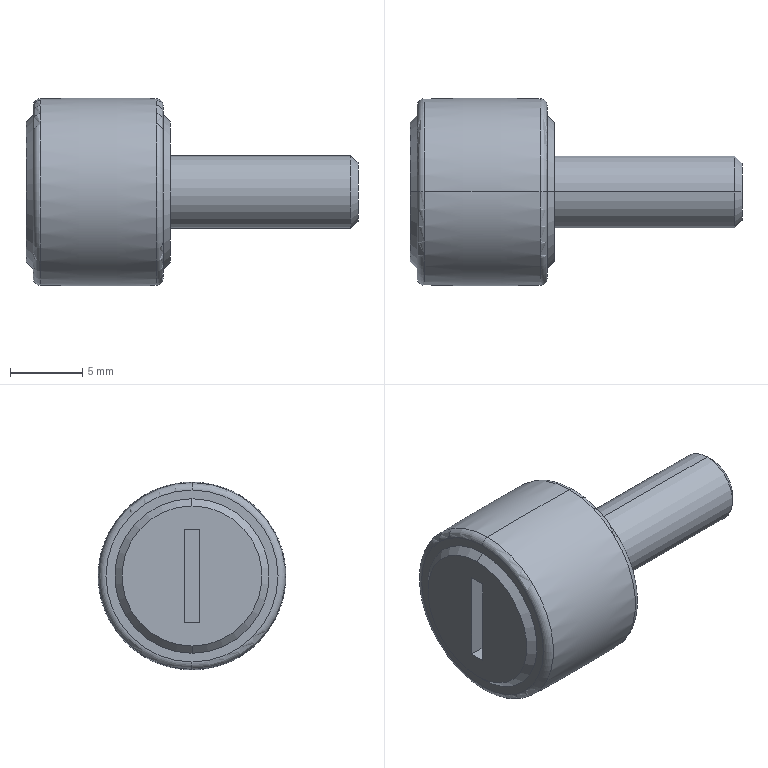Part | SolidWorks | features ICE 1, Revolution 1 | 1 solid | 24 faces | box 23 x 13 x 13 mm | volume 1507 mm3 | plane 10 | cone 6 | torus 6 | cylinder 2 | commonest cylinder face diameters 5 x2
STEP:
#1=CARTESIAN_POINT('',(13.,0.,2.01));
#2=VERTEX_POINT('',#1);
#3=CARTESIAN_POINT('',(13.,0.,-2.01));
#4=VERTEX_POINT('',#3);
#5=CARTESIAN_POINT('',(13.,0.,0.));
#6=DIRECTION('',(-1.,0.,0.));
#7=DIRECTION('',(0.,0.,1.));
#8=AXIS2_PLACEMENT_3D('',#5,#6,#7);
#9=CIRCLE('',#8,2.01);
#10=EDGE_CURVE('',#2,#4,#9,.T.);
#11=ORIENTED_EDGE('',*,*,#10,.T.);
#12=CARTESIAN_POINT('',(12.509,0.,-2.5));
#13=VERTEX_POINT('',#12);
#14=CARTESIAN_POINT('',(13.,0.,-2.01));
#15=DIRECTION('',(-0.7071,0.,-0.7071));
#16=VECTOR('',#15,1000.);
#17=LINE('',#14,#16);
#18=EDGE_CURVE('',#4,#13,#17,.T.);
#19=ORIENTED_EDGE('',*,*,#18,.T.);
#20=CARTESIAN_POINT('',(12.509,0.,2.5));
#21=VERTEX_POINT('',#20);
#22=CARTESIAN_POINT('',(12.509,0.,0.));
#23=DIRECTION('',(-1.,0.,0.));
#24=DIRECTION('',(0.,0.,1.));
#25=AXIS2_PLACEMENT_3D('',#22,#23,#24);
#26=CIRCLE('',#25,2.5);
#27=EDGE_CURVE('',#21,#13,#26,.T.);
#28=ORIENTED_EDGE('',*,*,#27,.F.);
#29=CARTESIAN_POINT('',(13.,0.,2.01));
#30=DIRECTION('',(-0.7071,0.,0.7071));
#31=VECTOR('',#30,1000.);
#32=LINE('',#29,#31);
#33=EDGE_CURVE('',#2,#21,#32,.T.);
#34=ORIENTED_EDGE('',*,*,#33,.F.);
#35=EDGE_LOOP('',(#11,#19,#28,#34));
#36=FACE_OUTER_BOUND('',#35,.T.);
#37=CARTESIAN_POINT('',(13.,0.,0.));
#38=DIRECTION('',(-1.,0.,0.));
#39=DIRECTION('',(0.,0.,1.));
#40=AXIS2_PLACEMENT_3D('',#37,#38,#39);
#41=CONICAL_SURFACE('',#40,2.01,0.7854);
#42=ADVANCED_FACE('',(#36),#41,.T.);
#43=ORIENTED_EDGE('',*,*,#27,.T.);
#44=CARTESIAN_POINT('',(0.,0.,-2.5));
#45=VERTEX_POINT('',#44);
#46=CARTESIAN_POINT('',(13.,0.,-2.5));
#47=DIRECTION('',(-1.,0.,0.));
#48=VECTOR('',#47,1000.);
#49=LINE('',#46,#48);
#50=EDGE_CURVE('',#13,#45,#49,.T.);
#51=ORIENTED_EDGE('',*,*,#50,.T.);
#52=CARTESIAN_POINT('',(0.,0.,2.5));
#53=VERTEX_POINT('',#52);
#54=CARTESIAN_POINT('',(0.,0.,0.));
#55=DIRECTION('',(-1.,0.,0.));
#56=DIRECTION('',(0.,0.,1.));
#57=AXIS2_PLACEMENT_3D('',#54,#55,#56);
#58=CIRCLE('',#57,2.5);
#59=EDGE_CURVE('',#53,#45,#58,.T.);
#60=ORIENTED_EDGE('',*,*,#59,.F.);
#61=CARTESIAN_POINT('',(13.,0.,2.5));
#62=DIRECTION('',(-1.,0.,0.));
#63=VECTOR('',#62,1000.);
#64=LINE('',#61,#63);
#65=EDGE_CURVE('',#21,#53,#64,.T.);
#66=ORIENTED_EDGE('',*,*,#65,.F.);
#67=EDGE_LOOP('',(#43,#51,#60,#66));
#68=FACE_OUTER_BOUND('',#67,.T.);
#69=CARTESIAN_POINT('',(13.,0.,0.));
#70=DIRECTION('',(-1.,0.,0.));
#71=DIRECTION('',(0.,0.,1.));
#72=AXIS2_PLACEMENT_3D('',#69,#70,#71);
#73=CYLINDRICAL_SURFACE('',#72,2.5);
#74=ADVANCED_FACE('',(#68),#73,.T.);
#75=CARTESIAN_POINT('',(0.,0.,4.85));
#76=VERTEX_POINT('',#75);
#77=CARTESIAN_POINT('',(0.,0.,-4.85));
#78=VERTEX_POINT('',#77);
#79=CARTESIAN_POINT('',(0.,0.,0.));
#80=DIRECTION('',(-1.,0.,0.));
#81=DIRECTION('',(0.,0.,1.));
#82=AXIS2_PLACEMENT_3D('',#79,#80,#81);
#83=CIRCLE('',#82,4.85);
#84=EDGE_CURVE('',#76,#78,#83,.T.);
#85=ORIENTED_EDGE('',*,*,#84,.T.);
#86=CARTESIAN_POINT('',(-0.5,0.,-5.35));
#87=VERTEX_POINT('',#86);
#88=CARTESIAN_POINT('',(0.,0.,-4.85));
#89=DIRECTION('',(-0.7071,0.,-0.7071));
#90=VECTOR('',#89,1000.);
#91=LINE('',#88,#90);
#92=EDGE_CURVE('',#78,#87,#91,.T.);
#93=ORIENTED_EDGE('',*,*,#92,.T.);
#94=CARTESIAN_POINT('',(-0.5,0.,5.35));
#95=VERTEX_POINT('',#94);
#96=CARTESIAN_POINT('',(-0.5,0.,0.));
#97=DIRECTION('',(-1.,0.,0.));
#98=DIRECTION('',(0.,0.,1.));
#99=AXIS2_PLACEMENT_3D('',#96,#97,#98);
#100=CIRCLE('',#99,5.35);
#101=EDGE_CURVE('',#95,#87,#100,.T.);
#102=ORIENTED_EDGE('',*,*,#101,.F.);
#103=CARTESIAN_POINT('',(0.,0.,4.85));
#104=DIRECTION('',(-0.7071,0.,0.7071));
#105=VECTOR('',#104,1000.);
#106=LINE('',#103,#105);
#107=EDGE_CURVE('',#76,#95,#106,.T.);
#108=ORIENTED_EDGE('',*,*,#107,.F.);
#109=EDGE_LOOP('',(#85,#93,#102,#108));
#110=FACE_OUTER_BOUND('',#109,.T.);
#111=CARTESIAN_POINT('',(0.,0.,0.));
#112=DIRECTION('',(-1.,0.,0.));
#113=DIRECTION('',(0.,0.,1.));
#114=AXIS2_PLACEMENT_3D('',#111,#112,#113);
#115=CONICAL_SURFACE('',#114,4.85,0.7854);
#116=ADVANCED_FACE('',(#110),#115,.T.);
#117=CARTESIAN_POINT('',(-0.5,0.,5.975));
#118=VERTEX_POINT('',#117);
#119=CARTESIAN_POINT('',(-0.5,0.,-5.975));
#120=VERTEX_POINT('',#119);
#121=CARTESIAN_POINT('',(-0.5,0.,0.));
#122=DIRECTION('',(-1.,0.,0.));
#123=DIRECTION('',(0.,0.,1.));
#124=AXIS2_PLACEMENT_3D('',#121,#122,#123);
#125=CIRCLE('',#124,5.975);
#126=EDGE_CURVE('',#118,#120,#125,.T.);
#127=ORIENTED_EDGE('',*,*,#126,.T.);
#128=CARTESIAN_POINT('',(-0.993,0.,-6.475));
#129=VERTEX_POINT('',#128);
#130=CARTESIAN_POINT('',(-1.,0.,-5.975));
#131=DIRECTION('',(0.,1.,0.));
#132=DIRECTION('',(0.,0.,1.));
#133=AXIS2_PLACEMENT_3D('',#130,#131,#132);
#134=CIRCLE('',#133,0.5);
#135=EDGE_CURVE('',#120,#129,#134,.T.);
#136=ORIENTED_EDGE('',*,*,#135,.T.);
#137=CARTESIAN_POINT('',(-0.993,0.,6.475));
#138=VERTEX_POINT('',#137);
#139=CARTESIAN_POINT('',(-0.993,0.,0.));
#140=DIRECTION('',(-1.,0.,0.));
#141=DIRECTION('',(0.,0.,1.));
#142=AXIS2_PLACEMENT_3D('',#139,#140,#141);
#143=CIRCLE('',#142,6.475);
#144=EDGE_CURVE('',#138,#129,#143,.T.);
#145=ORIENTED_EDGE('',*,*,#144,.F.);
#146=CARTESIAN_POINT('',(-1.,0.,5.975));
#147=DIRECTION('',(0.,-1.,0.));
#148=DIRECTION('',(0.,0.,-1.));
#149=AXIS2_PLACEMENT_3D('',#146,#147,#148);
#150=CIRCLE('',#149,0.5);
#151=EDGE_CURVE('',#118,#138,#150,.T.);
#152=ORIENTED_EDGE('',*,*,#151,.F.);
#153=EDGE_LOOP('',(#127,#136,#145,#152));
#154=FACE_OUTER_BOUND('',#153,.T.);
#155=CARTESIAN_POINT('',(-1.,0.,0.));
#156=DIRECTION('',(-1.,0.,0.));
#157=DIRECTION('',(0.,0.,1.));
#158=AXIS2_PLACEMENT_3D('',#155,#156,#157);
#159=TOROIDAL_SURFACE('',#158,5.975,0.5);
#160=ADVANCED_FACE('',(#154),#159,.T.);
#161=ORIENTED_EDGE('',*,*,#144,.T.);
#162=CARTESIAN_POINT('',(-9.009,0.,-6.459));
#163=VERTEX_POINT('',#162);
#164=CARTESIAN_POINT('',(-4.5,0.,243.5));
#165=DIRECTION('',(0.,1.,0.));
#166=DIRECTION('',(0.,0.,1.));
#167=AXIS2_PLACEMENT_3D('',#164,#165,#166);
#168=CIRCLE('',#167,250.);
#169=EDGE_CURVE('',#129,#163,#168,.T.);
#170=ORIENTED_EDGE('',*,*,#169,.T.);
#171=CARTESIAN_POINT('',(-9.009,0.,6.459));
#172=VERTEX_POINT('',#171);
#173=CARTESIAN_POINT('',(-9.009,0.,0.));
#174=DIRECTION('',(-1.,0.,0.));
#175=DIRECTION('',(0.,0.,1.));
#176=AXIS2_PLACEMENT_3D('',#173,#174,#175);
#177=CIRCLE('',#176,6.459);
#178=EDGE_CURVE('',#172,#163,#177,.T.);
#179=ORIENTED_EDGE('',*,*,#178,.F.);
#180=CARTESIAN_POINT('',(-4.5,0.,-243.5));
#181=DIRECTION('',(0.,-1.,0.));
#182=DIRECTION('',(0.,0.,-1.));
#183=AXIS2_PLACEMENT_3D('',#180,#181,#182);
#184=CIRCLE('',#183,250.);
#185=EDGE_CURVE('',#138,#172,#184,.T.);
#186=ORIENTED_EDGE('',*,*,#185,.F.);
#187=EDGE_LOOP('',(#161,#170,#179,#186));
#188=FACE_OUTER_BOUND('',#187,.T.);
#189=CARTESIAN_POINT('',(-4.5,0.,0.));
#190=DIRECTION('',(-1.,0.,0.));
#191=DIRECTION('',(0.,0.,1.));
#192=AXIS2_PLACEMENT_3D('',#189,#190,#191);
#193=TOROIDAL_SURFACE('',#192,-243.5,250.);
#194=ADVANCED_FACE('',(#188),#193,.T.);
#195=ORIENTED_EDGE('',*,*,#178,.T.);
#196=CARTESIAN_POINT('',(-9.5,0.,-5.959));
#197=VERTEX_POINT('',#196);
#198=CARTESIAN_POINT('',(-9.,0.,-5.959));
#199=DIRECTION('',(0.,1.,0.));
#200=DIRECTION('',(0.,0.,1.));
#201=AXIS2_PLACEMENT_3D('',#198,#199,#200);
#202=CIRCLE('',#201,0.5);
#203=EDGE_CURVE('',#163,#197,#202,.T.);
#204=ORIENTED_EDGE('',*,*,#203,.T.);
#205=CARTESIAN_POINT('',(-9.5,0.,5.959));
#206=VERTEX_POINT('',#205);
#207=CARTESIAN_POINT('',(-9.5,0.,0.));
#208=DIRECTION('',(-1.,0.,0.));
#209=DIRECTION('',(0.,0.,1.));
#210=AXIS2_PLACEMENT_3D('',#207,#208,#209);
#211=CIRCLE('',#210,5.959);
#212=EDGE_CURVE('',#206,#197,#211,.T.);
#213=ORIENTED_EDGE('',*,*,#212,.F.);
#214=CARTESIAN_POINT('',(-9.,0.,5.959));
#215=DIRECTION('',(0.,-1.,0.));
#216=DIRECTION('',(0.,0.,-1.));
#217=AXIS2_PLACEMENT_3D('',#214,#215,#216);
#218=CIRCLE('',#217,0.5);
#219=EDGE_CURVE('',#172,#206,#218,.T.);
#220=ORIENTED_EDGE('',*,*,#219,.F.);
#221=EDGE_LOOP('',(#195,#204,#213,#220));
#222=FACE_OUTER_BOUND('',#221,.T.);
#223=CARTESIAN_POINT('',(-9.,0.,0.));
#224=DIRECTION('',(-1.,0.,0.));
#225=DIRECTION('',(0.,0.,1.));
#226=AXIS2_PLACEMENT_3D('',#223,#224,#225);
#227=TOROIDAL_SURFACE('',#226,5.959,0.5);
#228=ADVANCED_FACE('',(#222),#227,.T.);
#229=CARTESIAN_POINT('',(-10.,0.,4.85));
#230=VERTEX_POINT('',#229);
#231=CARTESIAN_POINT('',(-10.,0.,-4.85));
#232=VERTEX_POINT('',#231);
#233=CARTESIAN_POINT('',(-10.,0.,0.));
#234=DIRECTION('',(-1.,0.,0.));
#235=DIRECTION('',(0.,0.,1.));
#236=AXIS2_PLACEMENT_3D('',#233,#234,#235);
#237=CIRCLE('',#236,4.85);
#238=EDGE_CURVE('',#230,#232,#237,.T.);
#239=ORIENTED_EDGE('',*,*,#238,.F.);
#240=CARTESIAN_POINT('',(-9.5,0.,5.35));
#241=VERTEX_POINT('',#240);
#242=CARTESIAN_POINT('',(-9.5,0.,5.35));
#243=DIRECTION('',(0.7071,0.,0.7071));
#244=VECTOR('',#243,1000.);
#245=LINE('',#242,#244);
#246=EDGE_CURVE('',#230,#241,#245,.T.);
#247=ORIENTED_EDGE('',*,*,#246,.T.);
#248=CARTESIAN_POINT('',(-9.5,0.,-5.35));
#249=VERTEX_POINT('',#248);
#250=CARTESIAN_POINT('',(-9.5,0.,0.));
#251=DIRECTION('',(-1.,0.,0.));
#252=DIRECTION('',(0.,0.,1.));
#253=AXIS2_PLACEMENT_3D('',#250,#251,#252);
#254=CIRCLE('',#253,5.35);
#255=EDGE_CURVE('',#241,#249,#254,.T.);
#256=ORIENTED_EDGE('',*,*,#255,.T.);
#257=CARTESIAN_POINT('',(-9.5,0.,-5.35));
#258=DIRECTION('',(0.7071,0.,-0.7071));
#259=VECTOR('',#258,1000.);
#260=LINE('',#257,#259);
#261=EDGE_CURVE('',#232,#249,#260,.T.);
#262=ORIENTED_EDGE('',*,*,#261,.F.);
#263=EDGE_LOOP('',(#239,#247,#256,#262));
#264=FACE_OUTER_BOUND('',#263,.T.);
#265=CARTESIAN_POINT('',(-9.5,0.,0.));
#266=DIRECTION('',(1.,0.,0.));
#267=DIRECTION('',(0.,0.,-1.));
#268=AXIS2_PLACEMENT_3D('',#265,#266,#267);
#269=CONICAL_SURFACE('',#268,5.35,0.7854);
#270=ADVANCED_FACE('',(#264),#269,.T.);
#271=CARTESIAN_POINT('',(-10.,-0.5417,3.25));
#272=VERTEX_POINT('',#271);
#273=CARTESIAN_POINT('',(-10.,0.5417,3.25));
#274=VERTEX_POINT('',#273);
#275=CARTESIAN_POINT('',(-10.,-0.5417,3.25));
#276=DIRECTION('',(0.,1.,0.));
#277=VECTOR('',#276,1000.);
#278=LINE('',#275,#277);
#279=EDGE_CURVE('',#272,#274,#278,.T.);
#280=ORIENTED_EDGE('',*,*,#279,.F.);
#281=CARTESIAN_POINT('',(-10.,-0.5417,-3.25));
#282=VERTEX_POINT('',#281);
#283=CARTESIAN_POINT('',(-10.,-0.5417,-3.25));
#284=DIRECTION('',(0.,0.,1.));
#285=VECTOR('',#284,1000.);
#286=LINE('',#283,#285);
#287=EDGE_CURVE('',#282,#272,#286,.T.);
#288=ORIENTED_EDGE('',*,*,#287,.F.);
#289=CARTESIAN_POINT('',(-10.,0.5417,-3.25));
#290=VERTEX_POINT('',#289);
#291=CARTESIAN_POINT('',(-10.,0.5417,-3.25));
#292=DIRECTION('',(0.,-1.,0.));
#293=VECTOR('',#292,1000.);
#294=LINE('',#291,#293);
#295=EDGE_CURVE('',#290,#282,#294,.T.);
#296=ORIENTED_EDGE('',*,*,#295,.F.);
#297=CARTESIAN_POINT('',(-10.,0.5417,3.25));
#298=DIRECTION('',(0.,0.,-1.));
#299=VECTOR('',#298,1000.);
#300=LINE('',#297,#299);
#301=EDGE_CURVE('',#274,#290,#300,.T.);
#302=ORIENTED_EDGE('',*,*,#301,.F.);
#303=EDGE_LOOP('',(#280,#288,#296,#302));
#304=FACE_BOUND('',#303,.T.);
#305=CARTESIAN_POINT('',(-10.,0.,0.));
#306=DIRECTION('',(-1.,0.,0.));
#307=DIRECTION('',(0.,0.,1.));
#308=AXIS2_PLACEMENT_3D('',#305,#306,#307);
#309=CIRCLE('',#308,4.85);
#310=EDGE_CURVE('',#232,#230,#309,.T.);
#311=ORIENTED_EDGE('',*,*,#310,.T.);
#312=ORIENTED_EDGE('',*,*,#238,.T.);
#313=EDGE_LOOP('',(#311,#312));
#314=FACE_OUTER_BOUND('',#313,.T.);
#315=CARTESIAN_POINT('',(-10.,0.,0.));
#316=DIRECTION('',(1.,0.,0.));
#317=DIRECTION('',(0.,0.,-1.));
#318=AXIS2_PLACEMENT_3D('',#315,#316,#317);
#319=PLANE('',#318);
#320=ADVANCED_FACE('',(#304,#314),#319,.F.);
#321=ORIENTED_EDGE('',*,*,#246,.F.);
#322=ORIENTED_EDGE('',*,*,#310,.F.);
#323=ORIENTED_EDGE('',*,*,#261,.T.);
#324=CARTESIAN_POINT('',(-9.5,0.,0.));
#325=DIRECTION('',(-1.,0.,0.));
#326=DIRECTION('',(0.,0.,1.));
#327=AXIS2_PLACEMENT_3D('',#324,#325,#326);
#328=CIRCLE('',#327,5.35);
#329=EDGE_CURVE('',#249,#241,#328,.T.);
#330=ORIENTED_EDGE('',*,*,#329,.T.);
#331=EDGE_LOOP('',(#321,#322,#323,#330));
#332=FACE_OUTER_BOUND('',#331,.T.);
#333=CARTESIAN_POINT('',(-9.5,0.,0.));
#334=DIRECTION('',(1.,0.,0.));
#335=DIRECTION('',(0.,0.,-1.));
#336=AXIS2_PLACEMENT_3D('',#333,#334,#335);
#337=CONICAL_SURFACE('',#336,5.35,0.7854);
#338=ADVANCED_FACE('',(#332),#337,.T.);
#339=ORIENTED_EDGE('',*,*,#329,.F.);
#340=ORIENTED_EDGE('',*,*,#255,.F.);
#341=EDGE_LOOP('',(#339,#340));
#342=FACE_BOUND('',#341,.T.);
#343=ORIENTED_EDGE('',*,*,#212,.T.);
#344=CARTESIAN_POINT('',(-9.5,0.,0.));
#345=DIRECTION('',(-1.,0.,0.));
#346=DIRECTION('',(0.,0.,1.));
#347=AXIS2_PLACEMENT_3D('',#344,#345,#346);
#348=CIRCLE('',#347,5.959);
#349=EDGE_CURVE('',#197,#206,#348,.T.);
#350=ORIENTED_EDGE('',*,*,#349,.T.);
#351=EDGE_LOOP('',(#343,#350));
#352=FACE_OUTER_BOUND('',#351,.T.);
#353=CARTESIAN_POINT('',(-9.5,5.35,0.));
#354=DIRECTION('',(1.,0.,0.));
#355=DIRECTION('',(0.,0.,-1.));
#356=AXIS2_PLACEMENT_3D('',#353,#354,#355);
#357=PLANE('',#356);
#358=ADVANCED_FACE('',(#342,#352),#357,.F.);
#359=ORIENTED_EDGE('',*,*,#203,.F.);
#360=CARTESIAN_POINT('',(-9.009,0.,0.));
#361=DIRECTION('',(-1.,0.,0.));
#362=DIRECTION('',(0.,0.,1.));
#363=AXIS2_PLACEMENT_3D('',#360,#361,#362);
#364=CIRCLE('',#363,6.459);
#365=EDGE_CURVE('',#163,#172,#364,.T.);
#366=ORIENTED_EDGE('',*,*,#365,.T.);
#367=ORIENTED_EDGE('',*,*,#219,.T.);
#368=ORIENTED_EDGE('',*,*,#349,.F.);
#369=EDGE_LOOP('',(#359,#366,#367,#368));
#370=FACE_OUTER_BOUND('',#369,.T.);
#371=CARTESIAN_POINT('',(-9.,0.,0.));
#372=DIRECTION('',(-1.,0.,0.));
#373=DIRECTION('',(0.,0.,1.));
#374=AXIS2_PLACEMENT_3D('',#371,#372,#373);
#375=TOROIDAL_SURFACE('',#374,5.959,0.5);
#376=ADVANCED_FACE('',(#370),#375,.T.);
#377=ORIENTED_EDGE('',*,*,#169,.F.);
#378=CARTESIAN_POINT('',(-0.993,0.,0.));
#379=DIRECTION('',(-1.,0.,0.));
#380=DIRECTION('',(0.,0.,1.));
#381=AXIS2_PLACEMENT_3D('',#378,#379,#380);
#382=CIRCLE('',#381,6.475);
#383=EDGE_CURVE('',#129,#138,#382,.T.);
#384=ORIENTED_EDGE('',*,*,#383,.T.);
#385=ORIENTED_EDGE('',*,*,#185,.T.);
#386=ORIENTED_EDGE('',*,*,#365,.F.);
#387=EDGE_LOOP('',(#377,#384,#385,#386));
#388=FACE_OUTER_BOUND('',#387,.T.);
#389=CARTESIAN_POINT('',(-4.5,0.,0.));
#390=DIRECTION('',(-1.,0.,0.));
#391=DIRECTION('',(0.,0.,1.));
#392=AXIS2_PLACEMENT_3D('',#389,#390,#391);
#393=TOROIDAL_SURFACE('',#392,-243.5,250.);
#394=ADVANCED_FACE('',(#388),#393,.T.);
#395=ORIENTED_EDGE('',*,*,#135,.F.);
#396=CARTESIAN_POINT('',(-0.5,0.,0.));
#397=DIRECTION('',(-1.,0.,0.));
#398=DIRECTION('',(0.,0.,1.));
#399=AXIS2_PLACEMENT_3D('',#396,#397,#398);
#400=CIRCLE('',#399,5.975);
#401=EDGE_CURVE('',#120,#118,#400,.T.);
#402=ORIENTED_EDGE('',*,*,#401,.T.);
#403=ORIENTED_EDGE('',*,*,#151,.T.);
#404=ORIENTED_EDGE('',*,*,#383,.F.);
#405=EDGE_LOOP('',(#395,#402,#403,#404));
#406=FACE_OUTER_BOUND('',#405,.T.);
#407=CARTESIAN_POINT('',(-1.,0.,0.));
#408=DIRECTION('',(-1.,0.,0.));
#409=DIRECTION('',(0.,0.,1.));
#410=AXIS2_PLACEMENT_3D('',#407,#408,#409);
#411=TOROIDAL_SURFACE('',#410,5.975,0.5);
#412=ADVANCED_FACE('',(#406),#411,.T.);
#413=ORIENTED_EDGE('',*,*,#126,.F.);
#414=ORIENTED_EDGE('',*,*,#401,.F.);
#415=EDGE_LOOP('',(#413,#414));
#416=FACE_OUTER_BOUND('',#415,.T.);
#417=ORIENTED_EDGE('',*,*,#101,.T.);
#418=CARTESIAN_POINT('',(-0.5,0.,0.));
#419=DIRECTION('',(-1.,0.,0.));
#420=DIRECTION('',(0.,0.,1.));
#421=AXIS2_PLACEMENT_3D('',#418,#419,#420);
#422=CIRCLE('',#421,5.35);
#423=EDGE_CURVE('',#87,#95,#422,.T.);
#424=ORIENTED_EDGE('',*,*,#423,.T.);
#425=EDGE_LOOP('',(#417,#424));
#426=FACE_BOUND('',#425,.T.);
#427=CARTESIAN_POINT('',(-0.5,5.975,0.));
#428=DIRECTION('',(-1.,0.,0.));
#429=DIRECTION('',(0.,0.,1.));
#430=AXIS2_PLACEMENT_3D('',#427,#428,#429);
#431=PLANE('',#430);
#432=ADVANCED_FACE('',(#416,#426),#431,.F.);
#433=ORIENTED_EDGE('',*,*,#92,.F.);
#434=CARTESIAN_POINT('',(0.,0.,0.));
#435=DIRECTION('',(-1.,0.,0.));
#436=DIRECTION('',(0.,0.,1.));
#437=AXIS2_PLACEMENT_3D('',#434,#435,#436);
#438=CIRCLE('',#437,4.85);
#439=EDGE_CURVE('',#78,#76,#438,.T.);
#440=ORIENTED_EDGE('',*,*,#439,.T.);
#441=ORIENTED_EDGE('',*,*,#107,.T.);
#442=ORIENTED_EDGE('',*,*,#423,.F.);
#443=EDGE_LOOP('',(#433,#440,#441,#442));
#444=FACE_OUTER_BOUND('',#443,.T.);
#445=CARTESIAN_POINT('',(0.,0.,0.));
#446=DIRECTION('',(-1.,0.,0.));
#447=DIRECTION('',(0.,0.,1.));
#448=AXIS2_PLACEMENT_3D('',#445,#446,#447);
#449=CONICAL_SURFACE('',#448,4.85,0.7854);
#450=ADVANCED_FACE('',(#444),#449,.T.);
#451=ORIENTED_EDGE('',*,*,#84,.F.);
#452=ORIENTED_EDGE('',*,*,#439,.F.);
#453=EDGE_LOOP('',(#451,#452));
#454=FACE_OUTER_BOUND('',#453,.T.);
#455=ORIENTED_EDGE('',*,*,#59,.T.);
#456=CARTESIAN_POINT('',(0.,0.,0.));
#457=DIRECTION('',(-1.,0.,0.));
#458=DIRECTION('',(0.,0.,1.));
#459=AXIS2_PLACEMENT_3D('',#456,#457,#458);
#460=CIRCLE('',#459,2.5);
#461=EDGE_CURVE('',#45,#53,#460,.T.);
#462=ORIENTED_EDGE('',*,*,#461,.T.);
#463=EDGE_LOOP('',(#455,#462));
#464=FACE_BOUND('',#463,.T.);
#465=CARTESIAN_POINT('',(0.,4.85,0.));
#466=DIRECTION('',(-1.,0.,0.));
#467=DIRECTION('',(0.,0.,1.));
#468=AXIS2_PLACEMENT_3D('',#465,#466,#467);
#469=PLANE('',#468);
#470=ADVANCED_FACE('',(#454,#464),#469,.F.);
#471=ORIENTED_EDGE('',*,*,#50,.F.);
#472=CARTESIAN_POINT('',(12.509,0.,0.));
#473=DIRECTION('',(-1.,0.,0.));
#474=DIRECTION('',(0.,0.,1.));
#475=AXIS2_PLACEMENT_3D('',#472,#473,#474);
#476=CIRCLE('',#475,2.5);
#477=EDGE_CURVE('',#13,#21,#476,.T.);
#478=ORIENTED_EDGE('',*,*,#477,.T.);
#479=ORIENTED_EDGE('',*,*,#65,.T.);
#480=ORIENTED_EDGE('',*,*,#461,.F.);
#481=EDGE_LOOP('',(#471,#478,#479,#480));
#482=FACE_OUTER_BOUND('',#481,.T.);
#483=CARTESIAN_POINT('',(13.,0.,0.));
#484=DIRECTION('',(-1.,0.,0.));
#485=DIRECTION('',(0.,0.,1.));
#486=AXIS2_PLACEMENT_3D('',#483,#484,#485);
#487=CYLINDRICAL_SURFACE('',#486,2.5);
#488=ADVANCED_FACE('',(#482),#487,.T.);
#489=ORIENTED_EDGE('',*,*,#18,.F.);
#490=CARTESIAN_POINT('',(13.,0.,0.));
#491=DIRECTION('',(-1.,0.,0.));
#492=DIRECTION('',(0.,0.,1.));
#493=AXIS2_PLACEMENT_3D('',#490,#491,#492);
#494=CIRCLE('',#493,2.01);
#495=EDGE_CURVE('',#4,#2,#494,.T.);
#496=ORIENTED_EDGE('',*,*,#495,.T.);
#497=ORIENTED_EDGE('',*,*,#33,.T.);
#498=ORIENTED_EDGE('',*,*,#477,.F.);
#499=EDGE_LOOP('',(#489,#496,#497,#498));
#500=FACE_OUTER_BOUND('',#499,.T.);
#501=CARTESIAN_POINT('',(13.,0.,0.));
#502=DIRECTION('',(-1.,0.,0.));
#503=DIRECTION('',(0.,0.,1.));
#504=AXIS2_PLACEMENT_3D('',#501,#502,#503);
#505=CONICAL_SURFACE('',#504,2.01,0.7854);
#506=ADVANCED_FACE('',(#500),#505,.T.);
#507=ORIENTED_EDGE('',*,*,#10,.F.);
#508=ORIENTED_EDGE('',*,*,#495,.F.);
#509=EDGE_LOOP('',(#507,#508));
#510=FACE_OUTER_BOUND('',#509,.T.);
#511=CARTESIAN_POINT('',(13.,2.01,0.));
#512=DIRECTION('',(-1.,0.,0.));
#513=DIRECTION('',(0.,0.,1.));
#514=AXIS2_PLACEMENT_3D('',#511,#512,#513);
#515=PLANE('',#514);
#516=ADVANCED_FACE('',(#510),#515,.F.);
#517=ORIENTED_EDGE('',*,*,#287,.T.);
#518=CARTESIAN_POINT('',(-8.,-0.5417,3.25));
#519=VERTEX_POINT('',#518);
#520=CARTESIAN_POINT('',(-8.,-0.5417,3.25));
#521=DIRECTION('',(-1.,0.,0.));
#522=VECTOR('',#521,1000.);
#523=LINE('',#520,#522);
#524=EDGE_CURVE('',#519,#272,#523,.T.);
#525=ORIENTED_EDGE('',*,*,#524,.F.);
#526=CARTESIAN_POINT('',(-8.,-0.5417,-3.25));
#527=VERTEX_POINT('',#526);
#528=CARTESIAN_POINT('',(-8.,-0.5417,-3.25));
#529=DIRECTION('',(0.,0.,1.));
#530=VECTOR('',#529,1000.);
#531=LINE('',#528,#530);
#532=EDGE_CURVE('',#527,#519,#531,.T.);
#533=ORIENTED_EDGE('',*,*,#532,.F.);
#534=CARTESIAN_POINT('',(-8.,-0.5417,-3.25));
#535=DIRECTION('',(-1.,0.,0.));
#536=VECTOR('',#535,1000.);
#537=LINE('',#534,#536);
#538=EDGE_CURVE('',#527,#282,#537,.T.);
#539=ORIENTED_EDGE('',*,*,#538,.T.);
#540=EDGE_LOOP('',(#517,#525,#533,#539));
#541=FACE_OUTER_BOUND('',#540,.T.);
#542=CARTESIAN_POINT('',(-8.,-0.5417,-3.25));
#543=DIRECTION('',(0.,-1.,0.));
#544=DIRECTION('',(0.,0.,-1.));
#545=AXIS2_PLACEMENT_3D('',#542,#543,#544);
#546=PLANE('',#545);
#547=ADVANCED_FACE('',(#541),#546,.F.);
#548=ORIENTED_EDGE('',*,*,#295,.T.);
#549=ORIENTED_EDGE('',*,*,#538,.F.);
#550=CARTESIAN_POINT('',(-8.,0.5417,-3.25));
#551=VERTEX_POINT('',#550);
#552=CARTESIAN_POINT('',(-8.,0.5417,-3.25));
#553=DIRECTION('',(0.,-1.,0.));
#554=VECTOR('',#553,1000.);
#555=LINE('',#552,#554);
#556=EDGE_CURVE('',#551,#527,#555,.T.);
#557=ORIENTED_EDGE('',*,*,#556,.F.);
#558=CARTESIAN_POINT('',(-8.,0.5417,-3.25));
#559=DIRECTION('',(-1.,0.,0.));
#560=VECTOR('',#559,1000.);
#561=LINE('',#558,#560);
#562=EDGE_CURVE('',#551,#290,#561,.T.);
#563=ORIENTED_EDGE('',*,*,#562,.T.);
#564=EDGE_LOOP('',(#548,#549,#557,#563));
#565=FACE_OUTER_BOUND('',#564,.T.);
#566=CARTESIAN_POINT('',(-8.,0.5417,-3.25));
#567=DIRECTION('',(0.,0.,-1.));
#568=DIRECTION('',(-1.,0.,0.));
#569=AXIS2_PLACEMENT_3D('',#566,#567,#568);
#570=PLANE('',#569);
#571=ADVANCED_FACE('',(#565),#570,.F.);
#572=ORIENTED_EDGE('',*,*,#301,.T.);
#573=ORIENTED_EDGE('',*,*,#562,.F.);
#574=CARTESIAN_POINT('',(-8.,0.5417,3.25));
#575=VERTEX_POINT('',#574);
#576=CARTESIAN_POINT('',(-8.,0.5417,3.25));
#577=DIRECTION('',(0.,0.,-1.));
#578=VECTOR('',#577,1000.);
#579=LINE('',#576,#578);
#580=EDGE_CURVE('',#575,#551,#579,.T.);
#581=ORIENTED_EDGE('',*,*,#580,.F.);
#582=CARTESIAN_POINT('',(-8.,0.5417,3.25));
#583=DIRECTION('',(-1.,0.,0.));
#584=VECTOR('',#583,1000.);
#585=LINE('',#582,#584);
#586=EDGE_CURVE('',#575,#274,#585,.T.);
#587=ORIENTED_EDGE('',*,*,#586,.T.);
#588=EDGE_LOOP('',(#572,#573,#581,#587));
#589=FACE_OUTER_BOUND('',#588,.T.);
#590=CARTESIAN_POINT('',(-8.,0.5417,3.25));
#591=DIRECTION('',(0.,1.,0.));
#592=DIRECTION('',(0.,0.,1.));
#593=AXIS2_PLACEMENT_3D('',#590,#591,#592);
#594=PLANE('',#593);
#595=ADVANCED_FACE('',(#589),#594,.F.);
#596=ORIENTED_EDGE('',*,*,#279,.T.);
#597=ORIENTED_EDGE('',*,*,#586,.F.);
#598=CARTESIAN_POINT('',(-8.,-0.5417,3.25));
#599=DIRECTION('',(0.,1.,0.));
#600=VECTOR('',#599,1000.);
#601=LINE('',#598,#600);
#602=EDGE_CURVE('',#519,#575,#601,.T.);
#603=ORIENTED_EDGE('',*,*,#602,.F.);
#604=ORIENTED_EDGE('',*,*,#524,.T.);
#605=EDGE_LOOP('',(#596,#597,#603,#604));
#606=FACE_OUTER_BOUND('',#605,.T.);
#607=CARTESIAN_POINT('',(-8.,-0.5417,3.25));
#608=DIRECTION('',(0.,0.,1.));
#609=DIRECTION('',(1.,0.,0.));
#610=AXIS2_PLACEMENT_3D('',#607,#608,#609);
#611=PLANE('',#610);
#612=ADVANCED_FACE('',(#606),#611,.F.);
#613=ORIENTED_EDGE('',*,*,#532,.T.);
#614=ORIENTED_EDGE('',*,*,#602,.T.);
#615=ORIENTED_EDGE('',*,*,#580,.T.);
#616=ORIENTED_EDGE('',*,*,#556,.T.);
#617=EDGE_LOOP('',(#613,#614,#615,#616));
#618=FACE_OUTER_BOUND('',#617,.T.);
#619=CARTESIAN_POINT('',(-8.,-0.5417,3.25));
#620=DIRECTION('',(-1.,0.,0.));
#621=DIRECTION('',(0.,0.,1.));
#622=AXIS2_PLACEMENT_3D('',#619,#620,#621);
#623=PLANE('',#622);
#624=ADVANCED_FACE('',(#618),#623,.T.);
#625=CLOSED_SHELL('',(#42,#74,#116,#160,#194,#228,#270,#320,#338,#358,#376,#394,#412,#432,#450,#470,#488,#506,#516,#547,#571,#595,#612,#624));
#626=MANIFOLD_SOLID_BREP('',#625);
#627=CARTESIAN_POINT('',(0.,0.,0.));
#628=DIRECTION('',(0.,0.,1.));
#629=DIRECTION('',(1.,0.,0.));
#630=AXIS2_PLACEMENT_3D('',#627,#628,#629);
#631=(LENGTH_UNIT()NAMED_UNIT(*)SI_UNIT(.MILLI.,.METRE.));
#632=UNCERTAINTY_MEASURE_WITH_UNIT(LENGTH_MEASURE(0.00001),#631,'','');
#633=(NAMED_UNIT(*)PLANE_ANGLE_UNIT()SI_UNIT($,.RADIAN.));
#634=(NAMED_UNIT(*)SI_UNIT($,.STERADIAN.)SOLID_ANGLE_UNIT());
#635=(GEOMETRIC_REPRESENTATION_CONTEXT(3)GLOBAL_UNCERTAINTY_ASSIGNED_CONTEXT((#632))GLOBAL_UNIT_ASSIGNED_CONTEXT((#631,#633,#634))REPRESENTATION_CONTEXT('',''));
#636=ADVANCED_BREP_SHAPE_REPRESENTATION('',(#626,#630),#635);